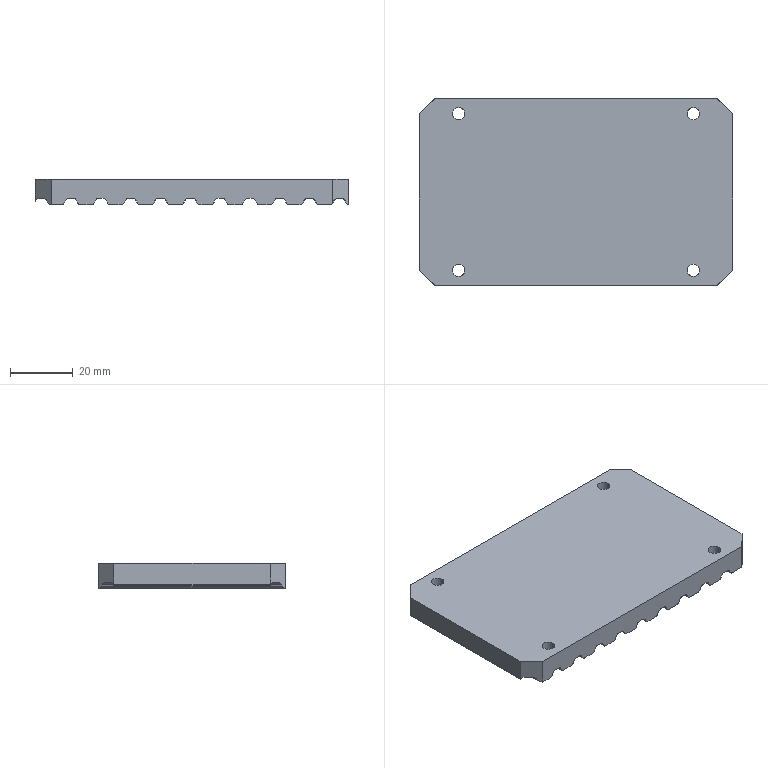Part | STEP file | Slider pressure plate | 1 solid | 119 faces | box 100 x 60 x 8 mm | volume 42576 mm3 | plane 60 | cylinder 59 | commonest cylinder face diameters 2.38 x28 2.34 x23 4 x8